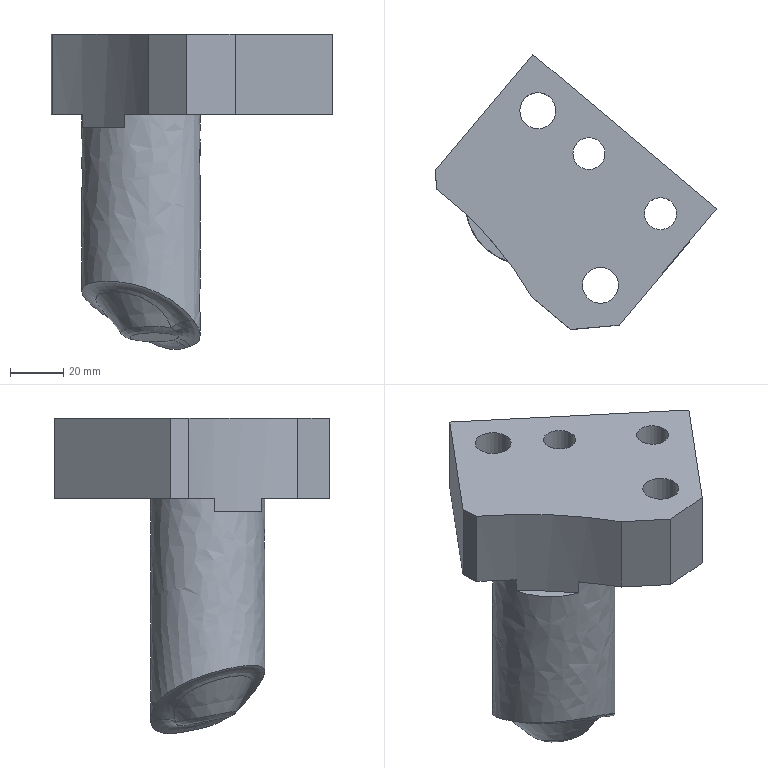Part | NX | features solid 2 | 1 solid | 26 faces | box 105.583 x 103.118 x 118.176 mm | volume 269895 mm3 | plane 12 | spline 8 | cylinder 6 | commonest cylinder face diameters 12 x2 13.5 x2 19.5 x2